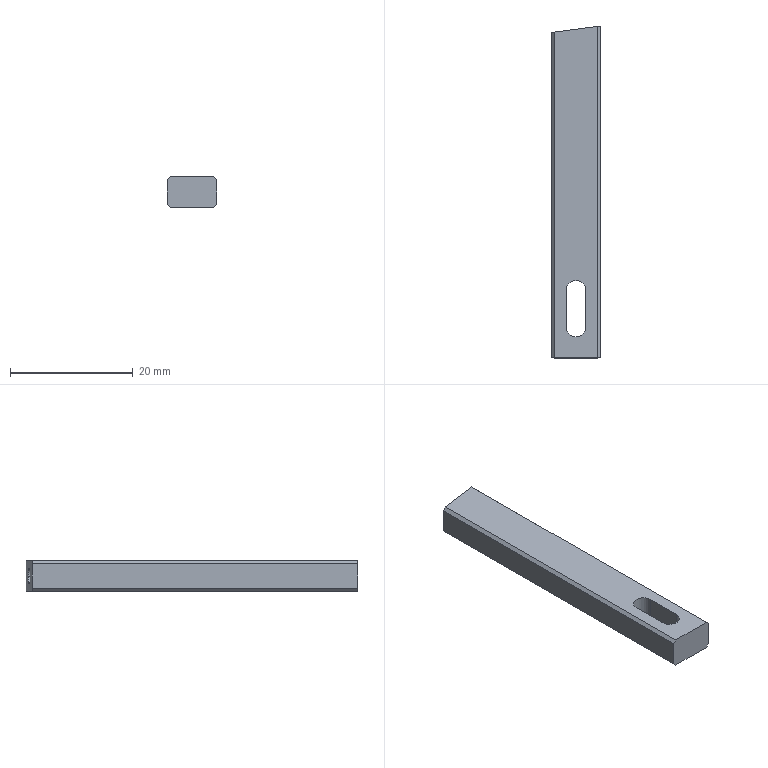Part | SolidWorks | features ICE 2, Chamfer 1, Extrusion 1, HoleWzd 1 | 1 solid | 18 faces | box 8 x 54 x 5 mm | volume 1933 mm3 | plane 12 | cylinder 4 | cone 2 | commonest cylinder face diameters 2.5 x2 3.2 x2